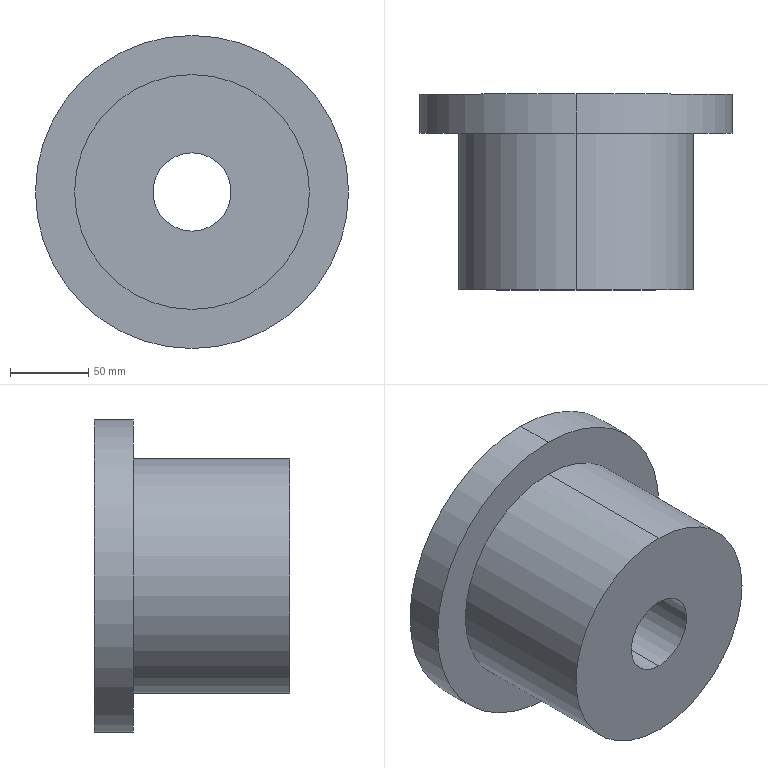Part | SolidWorks | features Revolution 1 | 1 solid | 9 faces | box 200 x 125 x 200 mm | volume 2307107 mm3 | cylinder 6 | plane 3 | commonest cylinder face diameters 50 x2 150 x2 200 x2
STEP:
#1=CARTESIAN_POINT('',(0.,-125.,75.));
#2=VERTEX_POINT('',#1);
#3=CARTESIAN_POINT('',(0.,-125.,-75.));
#4=VERTEX_POINT('',#3);
#5=CARTESIAN_POINT('',(0.,-125.,0.));
#6=DIRECTION('',(0.,1.,0.));
#7=DIRECTION('',(0.,0.,1.));
#8=AXIS2_PLACEMENT_3D('',#5,#6,#7);
#9=CIRCLE('',#8,75.);
#10=EDGE_CURVE('',#2,#4,#9,.T.);
#11=ORIENTED_EDGE('',*,*,#10,.T.);
#12=CARTESIAN_POINT('',(0.,-25.,-75.));
#13=VERTEX_POINT('',#12);
#14=CARTESIAN_POINT('',(0.,71.088,-75.));
#15=DIRECTION('',(0.,1.,0.));
#16=VECTOR('',#15,1000.);
#17=LINE('',#14,#16);
#18=EDGE_CURVE('',#4,#13,#17,.T.);
#19=ORIENTED_EDGE('',*,*,#18,.T.);
#20=CARTESIAN_POINT('',(0.,-25.,75.));
#21=VERTEX_POINT('',#20);
#22=CARTESIAN_POINT('',(0.,-25.,0.));
#23=DIRECTION('',(0.,1.,0.));
#24=DIRECTION('',(0.,0.,1.));
#25=AXIS2_PLACEMENT_3D('',#22,#23,#24);
#26=CIRCLE('',#25,75.);
#27=EDGE_CURVE('',#21,#13,#26,.T.);
#28=ORIENTED_EDGE('',*,*,#27,.F.);
#29=CARTESIAN_POINT('',(0.,71.088,75.));
#30=DIRECTION('',(0.,1.,0.));
#31=VECTOR('',#30,1000.);
#32=LINE('',#29,#31);
#33=EDGE_CURVE('',#2,#21,#32,.T.);
#34=ORIENTED_EDGE('',*,*,#33,.F.);
#35=EDGE_LOOP('',(#11,#19,#28,#34));
#36=FACE_OUTER_BOUND('',#35,.T.);
#37=CARTESIAN_POINT('',(0.,71.088,0.));
#38=DIRECTION('',(0.,1.,0.));
#39=DIRECTION('',(0.,0.,1.));
#40=AXIS2_PLACEMENT_3D('',#37,#38,#39);
#41=CYLINDRICAL_SURFACE('',#40,75.);
#42=ADVANCED_FACE('',(#36),#41,.T.);
#43=CARTESIAN_POINT('',(0.,-25.,100.));
#44=VERTEX_POINT('',#43);
#45=CARTESIAN_POINT('',(0.,-25.,-100.));
#46=VERTEX_POINT('',#45);
#47=CARTESIAN_POINT('',(0.,-25.,0.));
#48=DIRECTION('',(0.,1.,0.));
#49=DIRECTION('',(0.,0.,1.));
#50=AXIS2_PLACEMENT_3D('',#47,#48,#49);
#51=CIRCLE('',#50,100.);
#52=EDGE_CURVE('',#44,#46,#51,.T.);
#53=ORIENTED_EDGE('',*,*,#52,.T.);
#54=CARTESIAN_POINT('',(0.,0.,-100.));
#55=VERTEX_POINT('',#54);
#56=CARTESIAN_POINT('',(0.,71.088,-100.));
#57=DIRECTION('',(0.,1.,0.));
#58=VECTOR('',#57,1000.);
#59=LINE('',#56,#58);
#60=EDGE_CURVE('',#46,#55,#59,.T.);
#61=ORIENTED_EDGE('',*,*,#60,.T.);
#62=CARTESIAN_POINT('',(0.,0.,100.));
#63=VERTEX_POINT('',#62);
#64=CARTESIAN_POINT('',(0.,0.,0.));
#65=DIRECTION('',(0.,1.,0.));
#66=DIRECTION('',(0.,0.,1.));
#67=AXIS2_PLACEMENT_3D('',#64,#65,#66);
#68=CIRCLE('',#67,100.);
#69=EDGE_CURVE('',#63,#55,#68,.T.);
#70=ORIENTED_EDGE('',*,*,#69,.F.);
#71=CARTESIAN_POINT('',(0.,71.088,100.));
#72=DIRECTION('',(0.,1.,0.));
#73=VECTOR('',#72,1000.);
#74=LINE('',#71,#73);
#75=EDGE_CURVE('',#44,#63,#74,.T.);
#76=ORIENTED_EDGE('',*,*,#75,.F.);
#77=EDGE_LOOP('',(#53,#61,#70,#76));
#78=FACE_OUTER_BOUND('',#77,.T.);
#79=CARTESIAN_POINT('',(0.,71.088,0.));
#80=DIRECTION('',(0.,1.,0.));
#81=DIRECTION('',(0.,0.,1.));
#82=AXIS2_PLACEMENT_3D('',#79,#80,#81);
#83=CYLINDRICAL_SURFACE('',#82,100.);
#84=ADVANCED_FACE('',(#78),#83,.T.);
#85=CARTESIAN_POINT('',(0.,-125.,-25.));
#86=VERTEX_POINT('',#85);
#87=CARTESIAN_POINT('',(0.,-125.,25.));
#88=VERTEX_POINT('',#87);
#89=CARTESIAN_POINT('',(0.,-125.,0.));
#90=DIRECTION('',(0.,1.,0.));
#91=DIRECTION('',(0.,0.,1.));
#92=AXIS2_PLACEMENT_3D('',#89,#90,#91);
#93=CIRCLE('',#92,25.);
#94=EDGE_CURVE('',#86,#88,#93,.T.);
#95=ORIENTED_EDGE('',*,*,#94,.F.);
#96=CARTESIAN_POINT('',(0.,0.,-25.));
#97=VERTEX_POINT('',#96);
#98=CARTESIAN_POINT('',(0.,71.088,-25.));
#99=DIRECTION('',(0.,1.,0.));
#100=VECTOR('',#99,1000.);
#101=LINE('',#98,#100);
#102=EDGE_CURVE('',#86,#97,#101,.T.);
#103=ORIENTED_EDGE('',*,*,#102,.T.);
#104=CARTESIAN_POINT('',(0.,0.,25.));
#105=VERTEX_POINT('',#104);
#106=CARTESIAN_POINT('',(0.,0.,0.));
#107=DIRECTION('',(0.,1.,0.));
#108=DIRECTION('',(0.,0.,1.));
#109=AXIS2_PLACEMENT_3D('',#106,#107,#108);
#110=CIRCLE('',#109,25.);
#111=EDGE_CURVE('',#97,#105,#110,.T.);
#112=ORIENTED_EDGE('',*,*,#111,.T.);
#113=CARTESIAN_POINT('',(0.,71.088,25.));
#114=DIRECTION('',(0.,1.,0.));
#115=VECTOR('',#114,1000.);
#116=LINE('',#113,#115);
#117=EDGE_CURVE('',#88,#105,#116,.T.);
#118=ORIENTED_EDGE('',*,*,#117,.F.);
#119=EDGE_LOOP('',(#95,#103,#112,#118));
#120=FACE_OUTER_BOUND('',#119,.T.);
#121=CARTESIAN_POINT('',(0.,71.088,0.));
#122=DIRECTION('',(0.,1.,0.));
#123=DIRECTION('',(0.,0.,1.));
#124=AXIS2_PLACEMENT_3D('',#121,#122,#123);
#125=CYLINDRICAL_SURFACE('',#124,25.);
#126=ADVANCED_FACE('',(#120),#125,.F.);
#127=ORIENTED_EDGE('',*,*,#102,.F.);
#128=CARTESIAN_POINT('',(0.,-125.,0.));
#129=DIRECTION('',(0.,1.,0.));
#130=DIRECTION('',(0.,0.,1.));
#131=AXIS2_PLACEMENT_3D('',#128,#129,#130);
#132=CIRCLE('',#131,25.);
#133=EDGE_CURVE('',#88,#86,#132,.T.);
#134=ORIENTED_EDGE('',*,*,#133,.F.);
#135=ORIENTED_EDGE('',*,*,#117,.T.);
#136=CARTESIAN_POINT('',(0.,0.,0.));
#137=DIRECTION('',(0.,1.,0.));
#138=DIRECTION('',(0.,0.,1.));
#139=AXIS2_PLACEMENT_3D('',#136,#137,#138);
#140=CIRCLE('',#139,25.);
#141=EDGE_CURVE('',#105,#97,#140,.T.);
#142=ORIENTED_EDGE('',*,*,#141,.T.);
#143=EDGE_LOOP('',(#127,#134,#135,#142));
#144=FACE_OUTER_BOUND('',#143,.T.);
#145=CARTESIAN_POINT('',(0.,71.088,0.));
#146=DIRECTION('',(0.,1.,0.));
#147=DIRECTION('',(0.,0.,1.));
#148=AXIS2_PLACEMENT_3D('',#145,#146,#147);
#149=CYLINDRICAL_SURFACE('',#148,25.);
#150=ADVANCED_FACE('',(#144),#149,.F.);
#151=ORIENTED_EDGE('',*,*,#69,.T.);
#152=CARTESIAN_POINT('',(0.,0.,0.));
#153=DIRECTION('',(0.,1.,0.));
#154=DIRECTION('',(0.,0.,1.));
#155=AXIS2_PLACEMENT_3D('',#152,#153,#154);
#156=CIRCLE('',#155,100.);
#157=EDGE_CURVE('',#55,#63,#156,.T.);
#158=ORIENTED_EDGE('',*,*,#157,.T.);
#159=EDGE_LOOP('',(#151,#158));
#160=FACE_OUTER_BOUND('',#159,.T.);
#161=ORIENTED_EDGE('',*,*,#141,.F.);
#162=ORIENTED_EDGE('',*,*,#111,.F.);
#163=EDGE_LOOP('',(#161,#162));
#164=FACE_BOUND('',#163,.T.);
#165=CARTESIAN_POINT('',(-25.,0.,0.));
#166=DIRECTION('',(0.,1.,0.));
#167=DIRECTION('',(0.,0.,1.));
#168=AXIS2_PLACEMENT_3D('',#165,#166,#167);
#169=PLANE('',#168);
#170=ADVANCED_FACE('',(#160,#164),#169,.T.);
#171=ORIENTED_EDGE('',*,*,#60,.F.);
#172=CARTESIAN_POINT('',(0.,-25.,0.));
#173=DIRECTION('',(0.,1.,0.));
#174=DIRECTION('',(0.,0.,1.));
#175=AXIS2_PLACEMENT_3D('',#172,#173,#174);
#176=CIRCLE('',#175,100.);
#177=EDGE_CURVE('',#46,#44,#176,.T.);
#178=ORIENTED_EDGE('',*,*,#177,.T.);
#179=ORIENTED_EDGE('',*,*,#75,.T.);
#180=ORIENTED_EDGE('',*,*,#157,.F.);
#181=EDGE_LOOP('',(#171,#178,#179,#180));
#182=FACE_OUTER_BOUND('',#181,.T.);
#183=CARTESIAN_POINT('',(0.,71.088,0.));
#184=DIRECTION('',(0.,1.,0.));
#185=DIRECTION('',(0.,0.,1.));
#186=AXIS2_PLACEMENT_3D('',#183,#184,#185);
#187=CYLINDRICAL_SURFACE('',#186,100.);
#188=ADVANCED_FACE('',(#182),#187,.T.);
#189=ORIENTED_EDGE('',*,*,#27,.T.);
#190=CARTESIAN_POINT('',(0.,-25.,0.));
#191=DIRECTION('',(0.,1.,0.));
#192=DIRECTION('',(0.,0.,1.));
#193=AXIS2_PLACEMENT_3D('',#190,#191,#192);
#194=CIRCLE('',#193,75.);
#195=EDGE_CURVE('',#13,#21,#194,.T.);
#196=ORIENTED_EDGE('',*,*,#195,.T.);
#197=EDGE_LOOP('',(#189,#196));
#198=FACE_BOUND('',#197,.T.);
#199=ORIENTED_EDGE('',*,*,#52,.F.);
#200=ORIENTED_EDGE('',*,*,#177,.F.);
#201=EDGE_LOOP('',(#199,#200));
#202=FACE_OUTER_BOUND('',#201,.T.);
#203=CARTESIAN_POINT('',(-100.,-25.,0.));
#204=DIRECTION('',(0.,-1.,0.));
#205=DIRECTION('',(0.,0.,-1.));
#206=AXIS2_PLACEMENT_3D('',#203,#204,#205);
#207=PLANE('',#206);
#208=ADVANCED_FACE('',(#198,#202),#207,.T.);
#209=ORIENTED_EDGE('',*,*,#18,.F.);
#210=CARTESIAN_POINT('',(0.,-125.,0.));
#211=DIRECTION('',(0.,1.,0.));
#212=DIRECTION('',(0.,0.,1.));
#213=AXIS2_PLACEMENT_3D('',#210,#211,#212);
#214=CIRCLE('',#213,75.);
#215=EDGE_CURVE('',#4,#2,#214,.T.);
#216=ORIENTED_EDGE('',*,*,#215,.T.);
#217=ORIENTED_EDGE('',*,*,#33,.T.);
#218=ORIENTED_EDGE('',*,*,#195,.F.);
#219=EDGE_LOOP('',(#209,#216,#217,#218));
#220=FACE_OUTER_BOUND('',#219,.T.);
#221=CARTESIAN_POINT('',(0.,71.088,0.));
#222=DIRECTION('',(0.,1.,0.));
#223=DIRECTION('',(0.,0.,1.));
#224=AXIS2_PLACEMENT_3D('',#221,#222,#223);
#225=CYLINDRICAL_SURFACE('',#224,75.);
#226=ADVANCED_FACE('',(#220),#225,.T.);
#227=ORIENTED_EDGE('',*,*,#133,.T.);
#228=ORIENTED_EDGE('',*,*,#94,.T.);
#229=EDGE_LOOP('',(#227,#228));
#230=FACE_BOUND('',#229,.T.);
#231=ORIENTED_EDGE('',*,*,#10,.F.);
#232=ORIENTED_EDGE('',*,*,#215,.F.);
#233=EDGE_LOOP('',(#231,#232));
#234=FACE_OUTER_BOUND('',#233,.T.);
#235=CARTESIAN_POINT('',(-75.,-125.,0.));
#236=DIRECTION('',(0.,-1.,0.));
#237=DIRECTION('',(0.,0.,-1.));
#238=AXIS2_PLACEMENT_3D('',#235,#236,#237);
#239=PLANE('',#238);
#240=ADVANCED_FACE('',(#230,#234),#239,.T.);
#241=CLOSED_SHELL('',(#42,#84,#126,#150,#170,#188,#208,#226,#240));
#242=MANIFOLD_SOLID_BREP('',#241);
#243=CARTESIAN_POINT('',(0.,0.,0.));
#244=DIRECTION('',(0.,0.,1.));
#245=DIRECTION('',(1.,0.,0.));
#246=AXIS2_PLACEMENT_3D('',#243,#244,#245);
#247=(LENGTH_UNIT()NAMED_UNIT(*)SI_UNIT(.MILLI.,.METRE.));
#248=UNCERTAINTY_MEASURE_WITH_UNIT(LENGTH_MEASURE(0.00001),#247,'','');
#249=(NAMED_UNIT(*)PLANE_ANGLE_UNIT()SI_UNIT($,.RADIAN.));
#250=(NAMED_UNIT(*)SI_UNIT($,.STERADIAN.)SOLID_ANGLE_UNIT());
#251=(GEOMETRIC_REPRESENTATION_CONTEXT(3)GLOBAL_UNCERTAINTY_ASSIGNED_CONTEXT((#248))GLOBAL_UNIT_ASSIGNED_CONTEXT((#247,#249,#250))REPRESENTATION_CONTEXT('',''));
#252=ADVANCED_BREP_SHAPE_REPRESENTATION('',(#242,#246),#251);